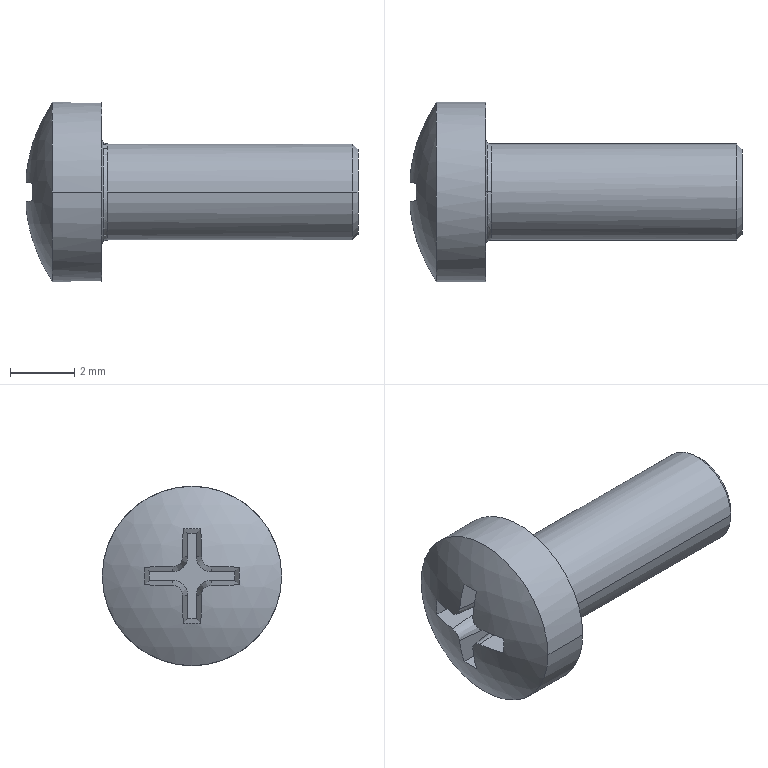Part | STEP file | ASSEMBLY_GB_T_9074_4_M3X8_1 | 1 solid | 30 faces | box 10.37 x 5.6 x 5.6 mm | volume 101.769 mm3 | plane 15 | cone 6 | cylinder 4 | torus 4 | sphere 1 | commonest cylinder face diameters 3 x2 5.6 x2